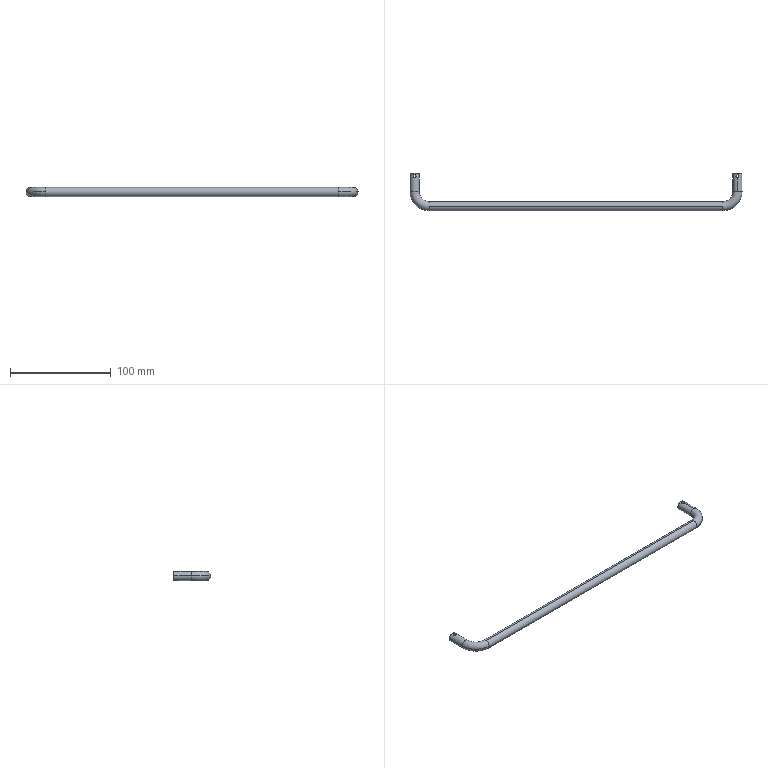Part | SolidWorks | features Chamfer 1, ICE 1, Sweep 1 | 1 solid | 20 faces | box 329 x 37 x 9 mm | volume 23569 mm3 | cylinder 10 | torus 4 | cone 4 | plane 2 | commonest cylinder face diameters 9 x6 3 x4
STEP:
#1=CARTESIAN_POINT('',(-4.5,-18.,0.));
#2=VERTEX_POINT('',#1);
#3=CARTESIAN_POINT('',(4.5,-18.,0.));
#4=VERTEX_POINT('',#3);
#5=CARTESIAN_POINT('',(0.,-18.,0.));
#6=DIRECTION('',(0.,1.,0.));
#7=DIRECTION('',(0.,0.,1.));
#8=AXIS2_PLACEMENT_3D('',#5,#6,#7);
#9=CIRCLE('',#8,4.5);
#10=EDGE_CURVE('',#2,#4,#9,.T.);
#11=ORIENTED_EDGE('',*,*,#10,.F.);
#12=CARTESIAN_POINT('',(14.5,-37.,0.));
#13=VERTEX_POINT('',#12);
#14=CARTESIAN_POINT('',(14.5,-18.,0.));
#15=DIRECTION('',(0.,0.,1.));
#16=DIRECTION('',(1.,0.,0.));
#17=AXIS2_PLACEMENT_3D('',#14,#15,#16);
#18=CIRCLE('',#17,19.);
#19=EDGE_CURVE('',#2,#13,#18,.T.);
#20=ORIENTED_EDGE('',*,*,#19,.T.);
#21=CARTESIAN_POINT('',(14.5,-32.5,4.5));
#22=VERTEX_POINT('',#21);
#23=CARTESIAN_POINT('',(14.5,-32.5,0.));
#24=DIRECTION('',(-1.,0.,0.));
#25=DIRECTION('',(0.,0.,1.));
#26=AXIS2_PLACEMENT_3D('',#23,#24,#25);
#27=CIRCLE('',#26,4.5);
#28=EDGE_CURVE('',#13,#22,#27,.T.);
#29=ORIENTED_EDGE('',*,*,#28,.T.);
#30=CARTESIAN_POINT('',(14.5,-28.,0.));
#31=VERTEX_POINT('',#30);
#32=CARTESIAN_POINT('',(14.5,-32.5,0.));
#33=DIRECTION('',(-1.,0.,0.));
#34=DIRECTION('',(0.,0.,1.));
#35=AXIS2_PLACEMENT_3D('',#32,#33,#34);
#36=CIRCLE('',#35,4.5);
#37=EDGE_CURVE('',#22,#31,#36,.T.);
#38=ORIENTED_EDGE('',*,*,#37,.T.);
#39=CARTESIAN_POINT('',(14.5,-18.,0.));
#40=DIRECTION('',(0.,0.,1.));
#41=DIRECTION('',(1.,0.,0.));
#42=AXIS2_PLACEMENT_3D('',#39,#40,#41);
#43=CIRCLE('',#42,10.);
#44=EDGE_CURVE('',#4,#31,#43,.T.);
#45=ORIENTED_EDGE('',*,*,#44,.F.);
#46=EDGE_LOOP('',(#11,#20,#29,#38,#45));
#47=FACE_OUTER_BOUND('',#46,.T.);
#48=CARTESIAN_POINT('',(14.5,-18.,0.));
#49=DIRECTION('',(0.,0.,1.));
#50=DIRECTION('',(1.,0.,0.));
#51=AXIS2_PLACEMENT_3D('',#48,#49,#50);
#52=TOROIDAL_SURFACE('',#51,14.5,4.5);
#53=ADVANCED_FACE('',(#47),#52,.T.);
#54=CARTESIAN_POINT('',(305.5,-37.,0.));
#55=VERTEX_POINT('',#54);
#56=CARTESIAN_POINT('',(305.5,-32.5,4.5));
#57=VERTEX_POINT('',#56);
#58=CARTESIAN_POINT('',(305.5,-32.5,0.));
#59=DIRECTION('',(-1.,0.,0.));
#60=DIRECTION('',(0.,0.,1.));
#61=AXIS2_PLACEMENT_3D('',#58,#59,#60);
#62=CIRCLE('',#61,4.5);
#63=EDGE_CURVE('',#55,#57,#62,.T.);
#64=ORIENTED_EDGE('',*,*,#63,.F.);
#65=CARTESIAN_POINT('',(324.5,-18.,0.));
#66=VERTEX_POINT('',#65);
#67=CARTESIAN_POINT('',(305.5,-18.,0.));
#68=DIRECTION('',(0.,0.,1.));
#69=DIRECTION('',(1.,0.,0.));
#70=AXIS2_PLACEMENT_3D('',#67,#68,#69);
#71=CIRCLE('',#70,19.);
#72=EDGE_CURVE('',#55,#66,#71,.T.);
#73=ORIENTED_EDGE('',*,*,#72,.T.);
#74=CARTESIAN_POINT('',(320.,-18.,4.5));
#75=VERTEX_POINT('',#74);
#76=CARTESIAN_POINT('',(320.,-18.,0.));
#77=DIRECTION('',(0.,-1.,0.));
#78=DIRECTION('',(0.,0.,1.));
#79=AXIS2_PLACEMENT_3D('',#76,#77,#78);
#80=CIRCLE('',#79,4.5);
#81=EDGE_CURVE('',#66,#75,#80,.T.);
#82=ORIENTED_EDGE('',*,*,#81,.T.);
#83=CARTESIAN_POINT('',(315.5,-18.,0.));
#84=VERTEX_POINT('',#83);
#85=CARTESIAN_POINT('',(320.,-18.,0.));
#86=DIRECTION('',(0.,-1.,0.));
#87=DIRECTION('',(0.,0.,1.));
#88=AXIS2_PLACEMENT_3D('',#85,#86,#87);
#89=CIRCLE('',#88,4.5);
#90=EDGE_CURVE('',#75,#84,#89,.T.);
#91=ORIENTED_EDGE('',*,*,#90,.T.);
#92=CARTESIAN_POINT('',(305.5,-28.,0.));
#93=VERTEX_POINT('',#92);
#94=CARTESIAN_POINT('',(305.5,-18.,0.));
#95=DIRECTION('',(0.,0.,1.));
#96=DIRECTION('',(1.,0.,0.));
#97=AXIS2_PLACEMENT_3D('',#94,#95,#96);
#98=CIRCLE('',#97,10.);
#99=EDGE_CURVE('',#93,#84,#98,.T.);
#100=ORIENTED_EDGE('',*,*,#99,.F.);
#101=CARTESIAN_POINT('',(305.5,-32.5,0.));
#102=DIRECTION('',(-1.,0.,0.));
#103=DIRECTION('',(0.,0.,1.));
#104=AXIS2_PLACEMENT_3D('',#101,#102,#103);
#105=CIRCLE('',#104,4.5);
#106=EDGE_CURVE('',#57,#93,#105,.T.);
#107=ORIENTED_EDGE('',*,*,#106,.F.);
#108=EDGE_LOOP('',(#64,#73,#82,#91,#100,#107));
#109=FACE_OUTER_BOUND('',#108,.T.);
#110=CARTESIAN_POINT('',(305.5,-18.,0.));
#111=DIRECTION('',(0.,0.,1.));
#112=DIRECTION('',(1.,0.,0.));
#113=AXIS2_PLACEMENT_3D('',#110,#111,#112);
#114=TOROIDAL_SURFACE('',#113,14.5,4.5);
#115=ADVANCED_FACE('',(#109),#114,.T.);
#116=CARTESIAN_POINT('',(-4.,0.,0.));
#117=VERTEX_POINT('',#116);
#118=CARTESIAN_POINT('',(4.,0.,0.));
#119=VERTEX_POINT('',#118);
#120=CARTESIAN_POINT('',(0.,0.,0.));
#121=DIRECTION('',(0.,1.,0.));
#122=DIRECTION('',(0.,0.,1.));
#123=AXIS2_PLACEMENT_3D('',#120,#121,#122);
#124=CIRCLE('',#123,4.);
#125=EDGE_CURVE('',#117,#119,#124,.T.);
#126=ORIENTED_EDGE('',*,*,#125,.F.);
#127=CARTESIAN_POINT('',(-4.5,-0.5,0.));
#128=VERTEX_POINT('',#127);
#129=CARTESIAN_POINT('',(-4.,0.,0.));
#130=DIRECTION('',(-0.7071,-0.7071,0.));
#131=VECTOR('',#130,1000.);
#132=LINE('',#129,#131);
#133=EDGE_CURVE('',#117,#128,#132,.T.);
#134=ORIENTED_EDGE('',*,*,#133,.T.);
#135=CARTESIAN_POINT('',(4.5,-0.5,0.));
#136=VERTEX_POINT('',#135);
#137=CARTESIAN_POINT('',(0.,-0.5,0.));
#138=DIRECTION('',(0.,-1.,0.));
#139=DIRECTION('',(-1.,0.,0.));
#140=AXIS2_PLACEMENT_3D('',#137,#138,#139);
#141=CIRCLE('',#140,4.5);
#142=EDGE_CURVE('',#136,#128,#141,.T.);
#143=ORIENTED_EDGE('',*,*,#142,.F.);
#144=CARTESIAN_POINT('',(4.,0.,0.));
#145=DIRECTION('',(0.7071,-0.7071,0.));
#146=VECTOR('',#145,1000.);
#147=LINE('',#144,#146);
#148=EDGE_CURVE('',#119,#136,#147,.T.);
#149=ORIENTED_EDGE('',*,*,#148,.F.);
#150=EDGE_LOOP('',(#126,#134,#143,#149));
#151=FACE_OUTER_BOUND('',#150,.T.);
#152=CARTESIAN_POINT('',(0.,0.,0.));
#153=DIRECTION('',(0.,-1.,0.));
#154=DIRECTION('',(1.,0.,0.));
#155=AXIS2_PLACEMENT_3D('',#152,#153,#154);
#156=CONICAL_SURFACE('',#155,4.,0.7854);
#157=ADVANCED_FACE('',(#151),#156,.T.);
#158=CARTESIAN_POINT('',(320.,0.,4.));
#159=VERTEX_POINT('',#158);
#160=CARTESIAN_POINT('',(320.,0.,-4.));
#161=VERTEX_POINT('',#160);
#162=CARTESIAN_POINT('',(320.,0.,0.));
#163=DIRECTION('',(0.,1.,0.));
#164=DIRECTION('',(1.,0.,0.));
#165=AXIS2_PLACEMENT_3D('',#162,#163,#164);
#166=CIRCLE('',#165,4.);
#167=EDGE_CURVE('',#159,#161,#166,.T.);
#168=ORIENTED_EDGE('',*,*,#167,.F.);
#169=CARTESIAN_POINT('',(320.,-0.5,4.5));
#170=VERTEX_POINT('',#169);
#171=CARTESIAN_POINT('',(320.,-0.5,4.5));
#172=DIRECTION('',(0.,-0.7071,0.7071));
#173=VECTOR('',#172,1000.);
#174=LINE('',#171,#173);
#175=EDGE_CURVE('',#159,#170,#174,.T.);
#176=ORIENTED_EDGE('',*,*,#175,.T.);
#177=CARTESIAN_POINT('',(320.,-0.5,-4.5));
#178=VERTEX_POINT('',#177);
#179=CARTESIAN_POINT('',(320.,-0.5,0.));
#180=DIRECTION('',(0.,-1.,0.));
#181=DIRECTION('',(0.,0.,-1.));
#182=AXIS2_PLACEMENT_3D('',#179,#180,#181);
#183=CIRCLE('',#182,4.5);
#184=EDGE_CURVE('',#178,#170,#183,.T.);
#185=ORIENTED_EDGE('',*,*,#184,.F.);
#186=CARTESIAN_POINT('',(320.,-0.5,-4.5));
#187=DIRECTION('',(0.,-0.7071,-0.7071));
#188=VECTOR('',#187,1000.);
#189=LINE('',#186,#188);
#190=EDGE_CURVE('',#161,#178,#189,.T.);
#191=ORIENTED_EDGE('',*,*,#190,.F.);
#192=EDGE_LOOP('',(#168,#176,#185,#191));
#193=FACE_OUTER_BOUND('',#192,.T.);
#194=CARTESIAN_POINT('',(320.,-0.5,0.));
#195=DIRECTION('',(0.,-1.,0.));
#196=DIRECTION('',(0.,0.,-1.));
#197=AXIS2_PLACEMENT_3D('',#194,#195,#196);
#198=CONICAL_SURFACE('',#197,4.5,0.7854);
#199=ADVANCED_FACE('',(#193),#198,.T.);
#200=CARTESIAN_POINT('',(1.5,-3.,4.243));
#201=VERTEX_POINT('',#200);
#202=CARTESIAN_POINT('',(-1.5,-3.,4.243));
#203=VERTEX_POINT('',#202);
#204=CARTESIAN_POINT('',(1.5,-3.,4.243));
#205=CARTESIAN_POINT('',(1.5,-3.197,4.243));
#206=CARTESIAN_POINT('',(1.46,-3.395,4.257));
#207=CARTESIAN_POINT('',(1.347,-3.667,4.294));
#208=CARTESIAN_POINT('',(1.3,-3.754,4.308));
#209=CARTESIAN_POINT('',(1.192,-3.916,4.34));
#210=CARTESIAN_POINT('',(1.13,-3.991,4.356));
#211=CARTESIAN_POINT('',(0.9222,-4.199,4.407));
#212=CARTESIAN_POINT('',(0.7586,-4.309,4.439));
#213=CARTESIAN_POINT('',(0.485,-4.423,4.475));
#214=CARTESIAN_POINT('',(0.3913,-4.451,4.484));
#215=CARTESIAN_POINT('',(0.1987,-4.49,4.497));
#216=CARTESIAN_POINT('',(0.09861,-4.5,4.5));
#217=CARTESIAN_POINT('',(-0.09905,-4.5,4.5));
#218=CARTESIAN_POINT('',(-0.1969,-4.49,4.497));
#219=CARTESIAN_POINT('',(-0.3908,-4.452,4.484));
#220=CARTESIAN_POINT('',(-0.4863,-4.422,4.475));
#221=CARTESIAN_POINT('',(-0.7573,-4.31,4.44));
#222=CARTESIAN_POINT('',(-0.9233,-4.198,4.407));
#223=CARTESIAN_POINT('',(-1.13,-3.992,4.357));
#224=CARTESIAN_POINT('',(-1.192,-3.915,4.34));
#225=CARTESIAN_POINT('',(-1.301,-3.753,4.308));
#226=CARTESIAN_POINT('',(-1.347,-3.667,4.294));
#227=CARTESIAN_POINT('',(-1.422,-3.486,4.269));
#228=CARTESIAN_POINT('',(-1.452,-3.391,4.259));
#229=CARTESIAN_POINT('',(-1.49,-3.198,4.246));
#230=CARTESIAN_POINT('',(-1.5,-3.1,4.243));
#231=CARTESIAN_POINT('',(-1.5,-3.,4.243));
#232=B_SPLINE_CURVE_WITH_KNOTS('',3,(#204,#205,#206,#207,#208,#209,#210,#211,#212,#213,#214,#215,#216,#217,#218,#219,#220,#221,#222,#223,#224,#225,#226,#227,#228,#229,#230,#231),.UNSPECIFIED.,.F.,.F.,(4,2,2,2,2,2,2,2,2,2,2,2,2,4),(0.004724,0.005314,0.005609,0.005904,0.006495,0.00679,0.007085,0.00738,0.007675,0.008265,0.008561,0.008856,0.009151,0.009446),.UNSPECIFIED.);
#233=EDGE_CURVE('',#201,#203,#232,.T.);
#234=ORIENTED_EDGE('',*,*,#233,.F.);
#235=CARTESIAN_POINT('',(1.5,-3.,-4.243));
#236=VERTEX_POINT('',#235);
#237=CARTESIAN_POINT('',(1.5,-3.,10.));
#238=DIRECTION('',(0.,0.,-1.));
#239=VECTOR('',#238,1000.);
#240=LINE('',#237,#239);
#241=EDGE_CURVE('',#201,#236,#240,.T.);
#242=ORIENTED_EDGE('',*,*,#241,.T.);
#243=CARTESIAN_POINT('',(-1.5,-3.,-4.243));
#244=VERTEX_POINT('',#243);
#245=CARTESIAN_POINT('',(-1.5,-3.,-4.243));
#246=CARTESIAN_POINT('',(-1.5,-3.1,-4.243));
#247=CARTESIAN_POINT('',(-1.49,-3.198,-4.246));
#248=CARTESIAN_POINT('',(-1.452,-3.391,-4.26));
#249=CARTESIAN_POINT('',(-1.422,-3.486,-4.269));
#250=CARTESIAN_POINT('',(-1.309,-3.758,-4.306));
#251=CARTESIAN_POINT('',(-1.198,-3.924,-4.34));
#252=CARTESIAN_POINT('',(-0.9231,-4.198,-4.407));
#253=CARTESIAN_POINT('',(-0.757,-4.31,-4.44));
#254=CARTESIAN_POINT('',(-0.3964,-4.46,-4.486));
#255=CARTESIAN_POINT('',(-0.198,-4.5,-4.5));
#256=CARTESIAN_POINT('',(0.09798,-4.5,-4.5));
#257=CARTESIAN_POINT('',(0.1982,-4.49,-4.497));
#258=CARTESIAN_POINT('',(0.3912,-4.451,-4.484));
#259=CARTESIAN_POINT('',(0.4851,-4.423,-4.475));
#260=CARTESIAN_POINT('',(0.759,-4.309,-4.439));
#261=CARTESIAN_POINT('',(0.9234,-4.198,-4.407));
#262=CARTESIAN_POINT('',(1.13,-3.991,-4.356));
#263=CARTESIAN_POINT('',(1.192,-3.916,-4.34));
#264=CARTESIAN_POINT('',(1.3,-3.754,-4.308));
#265=CARTESIAN_POINT('',(1.348,-3.666,-4.294));
#266=CARTESIAN_POINT('',(1.46,-3.395,-4.257));
#267=CARTESIAN_POINT('',(1.5,-3.197,-4.243));
#268=CARTESIAN_POINT('',(1.5,-3.,-4.243));
#269=B_SPLINE_CURVE_WITH_KNOTS('',3,(#245,#246,#247,#248,#249,#250,#251,#252,#253,#254,#255,#256,#257,#258,#259,#260,#261,#262,#263,#264,#265,#266,#267,#268),.UNSPECIFIED.,.F.,.F.,(4,2,2,2,2,2,2,2,2,2,2,4),(0.,0.0002952,0.0005905,0.001181,0.001771,0.002362,0.002657,0.002952,0.003543,0.003838,0.004133,0.004724),.UNSPECIFIED.);
#270=EDGE_CURVE('',#244,#236,#269,.T.);
#271=ORIENTED_EDGE('',*,*,#270,.F.);
#272=CARTESIAN_POINT('',(-1.5,-3.,10.));
#273=DIRECTION('',(0.,0.,-1.));
#274=VECTOR('',#273,1000.);
#275=LINE('',#272,#274);
#276=EDGE_CURVE('',#203,#244,#275,.T.);
#277=ORIENTED_EDGE('',*,*,#276,.F.);
#278=EDGE_LOOP('',(#234,#242,#271,#277));
#279=FACE_OUTER_BOUND('',#278,.T.);
#280=CARTESIAN_POINT('',(0.,-3.,10.));
#281=DIRECTION('',(0.,0.,-1.));
#282=DIRECTION('',(-1.,0.,0.));
#283=AXIS2_PLACEMENT_3D('',#280,#281,#282);
#284=CYLINDRICAL_SURFACE('',#283,1.5);
#285=ADVANCED_FACE('',(#279),#284,.F.);
#286=CARTESIAN_POINT('',(320.,-4.5,4.5));
#287=VERTEX_POINT('',#286);
#288=CARTESIAN_POINT('',(321.5,-3.,4.243));
#289=VERTEX_POINT('',#288);
#290=CARTESIAN_POINT('',(320.,-4.5,4.5));
#291=CARTESIAN_POINT('',(320.1,-4.5,4.5));
#292=CARTESIAN_POINT('',(320.198,-4.49,4.497));
#293=CARTESIAN_POINT('',(320.391,-4.452,4.484));
#294=CARTESIAN_POINT('',(320.486,-4.422,4.475));
#295=CARTESIAN_POINT('',(320.759,-4.309,4.439));
#296=CARTESIAN_POINT('',(320.924,-4.197,4.406));
#297=CARTESIAN_POINT('',(321.199,-3.922,4.34));
#298=CARTESIAN_POINT('',(321.31,-3.756,4.306));
#299=CARTESIAN_POINT('',(321.46,-3.396,4.257));
#300=CARTESIAN_POINT('',(321.5,-3.197,4.243));
#301=CARTESIAN_POINT('',(321.5,-3.,4.243));
#302=B_SPLINE_CURVE_WITH_KNOTS('',3,(#290,#291,#292,#293,#294,#295,#296,#297,#298,#299,#300,#301),.UNSPECIFIED.,.F.,.F.,(4,2,2,2,2,4),(0.,0.0002953,0.0005907,0.001181,0.001772,0.002363),.UNSPECIFIED.);
#303=EDGE_CURVE('',#287,#289,#302,.T.);
#304=ORIENTED_EDGE('',*,*,#303,.T.);
#305=CARTESIAN_POINT('',(321.5,-3.,-4.243));
#306=VERTEX_POINT('',#305);
#307=CARTESIAN_POINT('',(321.5,-3.,10.));
#308=DIRECTION('',(0.,0.,-1.));
#309=VECTOR('',#308,1000.);
#310=LINE('',#307,#309);
#311=EDGE_CURVE('',#289,#306,#310,.T.);
#312=ORIENTED_EDGE('',*,*,#311,.T.);
#313=CARTESIAN_POINT('',(320.,-4.5,-4.5));
#314=VERTEX_POINT('',#313);
#315=CARTESIAN_POINT('',(321.5,-3.,-4.243));
#316=CARTESIAN_POINT('',(321.5,-3.197,-4.243));
#317=CARTESIAN_POINT('',(321.46,-3.395,-4.257));
#318=CARTESIAN_POINT('',(321.347,-3.667,-4.294));
#319=CARTESIAN_POINT('',(321.3,-3.754,-4.308));
#320=CARTESIAN_POINT('',(321.192,-3.916,-4.34));
#321=CARTESIAN_POINT('',(321.13,-3.991,-4.356));
#322=CARTESIAN_POINT('',(320.922,-4.199,-4.407));
#323=CARTESIAN_POINT('',(320.759,-4.309,-4.439));
#324=CARTESIAN_POINT('',(320.485,-4.423,-4.475));
#325=CARTESIAN_POINT('',(320.391,-4.451,-4.484));
#326=CARTESIAN_POINT('',(320.199,-4.49,-4.497));
#327=CARTESIAN_POINT('',(320.099,-4.5,-4.5));
#328=CARTESIAN_POINT('',(320.,-4.5,-4.5));
#329=B_SPLINE_CURVE_WITH_KNOTS('',3,(#315,#316,#317,#318,#319,#320,#321,#322,#323,#324,#325,#326,#327,#328),.UNSPECIFIED.,.F.,.F.,(4,2,2,2,2,2,4),(0.004724,0.005314,0.005609,0.005904,0.006494,0.006789,0.007085),.UNSPECIFIED.);
#330=EDGE_CURVE('',#306,#314,#329,.T.);
#331=ORIENTED_EDGE('',*,*,#330,.T.);
#332=CARTESIAN_POINT('',(318.5,-3.,-4.243));
#333=VERTEX_POINT('',#332);
#334=CARTESIAN_POINT('',(320.,-4.5,-4.5));
#335=CARTESIAN_POINT('',(319.901,-4.5,-4.5));
#336=CARTESIAN_POINT('',(319.803,-4.49,-4.497));
#337=CARTESIAN_POINT('',(319.609,-4.452,-4.484));
#338=CARTESIAN_POINT('',(319.514,-4.422,-4.475));
#339=CARTESIAN_POINT('',(319.243,-4.31,-4.44));
#340=CARTESIAN_POINT('',(319.077,-4.198,-4.407));
#341=CARTESIAN_POINT('',(318.871,-3.992,-4.357));
#342=CARTESIAN_POINT('',(318.808,-3.915,-4.34));
#343=CARTESIAN_POINT('',(318.699,-3.753,-4.308));
#344=CARTESIAN_POINT('',(318.653,-3.667,-4.294));
#345=CARTESIAN_POINT('',(318.578,-3.486,-4.269));
#346=CARTESIAN_POINT('',(318.548,-3.391,-4.259));
#347=CARTESIAN_POINT('',(318.51,-3.198,-4.246));
#348=CARTESIAN_POINT('',(318.5,-3.1,-4.243));
#349=CARTESIAN_POINT('',(318.5,-3.,-4.243));
#350=B_SPLINE_CURVE_WITH_KNOTS('',3,(#334,#335,#336,#337,#338,#339,#340,#341,#342,#343,#344,#345,#346,#347,#348,#349),.UNSPECIFIED.,.F.,.F.,(4,2,2,2,2,2,2,4),(0.007085,0.00738,0.007675,0.008265,0.00856,0.008856,0.009151,0.009446),.UNSPECIFIED.);
#351=EDGE_CURVE('',#314,#333,#350,.T.);
#352=ORIENTED_EDGE('',*,*,#351,.T.);
#353=CARTESIAN_POINT('',(318.5,-3.,4.243));
#354=VERTEX_POINT('',#353);
#355=CARTESIAN_POINT('',(318.5,-3.,10.));
#356=DIRECTION('',(0.,0.,-1.));
#357=VECTOR('',#356,1000.);
#358=LINE('',#355,#357);
#359=EDGE_CURVE('',#354,#333,#358,.T.);
#360=ORIENTED_EDGE('',*,*,#359,.F.);
#361=CARTESIAN_POINT('',(318.5,-3.,4.243));
#362=CARTESIAN_POINT('',(318.5,-3.099,4.243));
#363=CARTESIAN_POINT('',(318.51,-3.197,4.246));
#364=CARTESIAN_POINT('',(318.548,-3.391,4.259));
#365=CARTESIAN_POINT('',(318.578,-3.486,4.269));
#366=CARTESIAN_POINT('',(318.69,-3.757,4.306));
#367=CARTESIAN_POINT('',(318.802,-3.923,4.34));
#368=CARTESIAN_POINT('',(319.008,-4.129,4.39));
#369=CARTESIAN_POINT('',(319.084,-4.192,4.407));
#370=CARTESIAN_POINT('',(319.247,-4.301,4.437));
#371=CARTESIAN_POINT('',(319.332,-4.347,4.451));
#372=CARTESIAN_POINT('',(319.514,-4.422,4.475));
#373=CARTESIAN_POINT('',(319.609,-4.452,4.484));
#374=CARTESIAN_POINT('',(319.802,-4.49,4.497));
#375=CARTESIAN_POINT('',(319.9,-4.5,4.5));
#376=CARTESIAN_POINT('',(320.,-4.5,4.5));
#377=B_SPLINE_CURVE_WITH_KNOTS('',3,(#361,#362,#363,#364,#365,#366,#367,#368,#369,#370,#371,#372,#373,#374,#375,#376),.UNSPECIFIED.,.F.,.F.,(4,2,2,2,2,2,2,4),(0.007085,0.00738,0.007675,0.008266,0.008561,0.008856,0.009151,0.009446),.UNSPECIFIED.);
#378=EDGE_CURVE('',#354,#287,#377,.T.);
#379=ORIENTED_EDGE('',*,*,#378,.T.);
#380=EDGE_LOOP('',(#304,#312,#331,#352,#360,#379));
#381=FACE_OUTER_BOUND('',#380,.T.);
#382=CARTESIAN_POINT('',(320.,-3.,10.));
#383=DIRECTION('',(0.,0.,-1.));
#384=DIRECTION('',(-1.,0.,0.));
#385=AXIS2_PLACEMENT_3D('',#382,#383,#384);
#386=CYLINDRICAL_SURFACE('',#385,1.5);
#387=ADVANCED_FACE('',(#381),#386,.F.);
#388=ORIENTED_EDGE('',*,*,#37,.F.);
#389=CARTESIAN_POINT('',(14.5,-32.5,4.5));
#390=DIRECTION('',(1.,0.,0.));
#391=VECTOR('',#390,1000.);
#392=LINE('',#389,#391);
#393=EDGE_CURVE('',#22,#57,#392,.T.);
#394=ORIENTED_EDGE('',*,*,#393,.T.);
#395=ORIENTED_EDGE('',*,*,#106,.T.);
#396=CARTESIAN_POINT('',(305.5,-32.5,-4.5));
#397=VERTEX_POINT('',#396);
#398=CARTESIAN_POINT('',(305.5,-32.5,0.));
#399=DIRECTION('',(-1.,0.,0.));
#400=DIRECTION('',(0.,0.,1.));
#401=AXIS2_PLACEMENT_3D('',#398,#399,#400);
#402=CIRCLE('',#401,4.5);
#403=EDGE_CURVE('',#93,#397,#402,.T.);
#404=ORIENTED_EDGE('',*,*,#403,.T.);
#405=CARTESIAN_POINT('',(14.5,-32.5,-4.5));
#406=VERTEX_POINT('',#405);
#407=CARTESIAN_POINT('',(14.5,-32.5,-4.5));
#408=DIRECTION('',(1.,0.,0.));
#409=VECTOR('',#408,1000.);
#410=LINE('',#407,#409);
#411=EDGE_CURVE('',#406,#397,#410,.T.);
#412=ORIENTED_EDGE('',*,*,#411,.F.);
#413=CARTESIAN_POINT('',(14.5,-32.5,0.));
#414=DIRECTION('',(-1.,0.,0.));
#415=DIRECTION('',(0.,0.,1.));
#416=AXIS2_PLACEMENT_3D('',#413,#414,#415);
#417=CIRCLE('',#416,4.5);
#418=EDGE_CURVE('',#31,#406,#417,.T.);
#419=ORIENTED_EDGE('',*,*,#418,.F.);
#420=EDGE_LOOP('',(#388,#394,#395,#404,#412,#419));
#421=FACE_OUTER_BOUND('',#420,.T.);
#422=CARTESIAN_POINT('',(14.5,-32.5,0.));
#423=DIRECTION('',(1.,0.,0.));
#424=DIRECTION('',(0.,0.,-1.));
#425=AXIS2_PLACEMENT_3D('',#422,#423,#424);
#426=CYLINDRICAL_SURFACE('',#425,4.5);
#427=ADVANCED_FACE('',(#421),#426,.T.);
#428=CARTESIAN_POINT('',(320.,-18.,-4.5));
#429=VERTEX_POINT('',#428);
#430=CARTESIAN_POINT('',(320.,-18.,0.));
#431=DIRECTION('',(0.,-1.,0.));
#432=DIRECTION('',(0.,0.,1.));
#433=AXIS2_PLACEMENT_3D('',#430,#431,#432);
#434=CIRCLE('',#433,4.5);
#435=EDGE_CURVE('',#429,#66,#434,.T.);
#436=ORIENTED_EDGE('',*,*,#435,.F.);
#437=CARTESIAN_POINT('',(320.,-18.,-4.5));
#438=DIRECTION('',(0.,1.,0.));
#439=VECTOR('',#438,1000.);
#440=LINE('',#437,#439);
#441=EDGE_CURVE('',#429,#314,#440,.T.);
#442=ORIENTED_EDGE('',*,*,#441,.T.);
#443=ORIENTED_EDGE('',*,*,#330,.F.);
#444=CARTESIAN_POINT('',(320.,-1.5,-4.5));
#445=VERTEX_POINT('',#444);
#446=CARTESIAN_POINT('',(320.,-1.5,-4.5));
#447=CARTESIAN_POINT('',(320.099,-1.5,-4.5));
#448=CARTESIAN_POINT('',(320.199,-1.51,-4.497));
#449=CARTESIAN_POINT('',(320.392,-1.549,-4.484));
#450=CARTESIAN_POINT('',(320.486,-1.577,-4.475));
#451=CARTESIAN_POINT('',(320.759,-1.691,-4.439));
#452=CARTESIAN_POINT('',(320.924,-1.802,-4.406));
#453=CARTESIAN_POINT('',(321.131,-2.009,-4.356));
#454=CARTESIAN_POINT('',(321.192,-2.084,-4.34));
#455=CARTESIAN_POINT('',(321.301,-2.246,-4.308));
#456=CARTESIAN_POINT('',(321.348,-2.334,-4.294));
#457=CARTESIAN_POINT('',(321.46,-2.605,-4.257));
#458=CARTESIAN_POINT('',(321.5,-2.803,-4.243));
#459=CARTESIAN_POINT('',(321.5,-3.,-4.243));
#460=B_SPLINE_CURVE_WITH_KNOTS('',3,(#446,#447,#448,#449,#450,#451,#452,#453,#454,#455,#456,#457,#458,#459),.UNSPECIFIED.,.F.,.F.,(4,2,2,2,2,2,4),(0.002362,0.002658,0.002953,0.003543,0.003838,0.004133,0.004724),.UNSPECIFIED.);
#461=EDGE_CURVE('',#445,#306,#460,.T.);
#462=ORIENTED_EDGE('',*,*,#461,.F.);
#463=CARTESIAN_POINT('',(320.,-18.,-4.5));
#464=DIRECTION('',(0.,1.,0.));
#465=VECTOR('',#464,1000.);
#466=LINE('',#463,#465);
#467=EDGE_CURVE('',#445,#178,#466,.T.);
#468=ORIENTED_EDGE('',*,*,#467,.T.);
#469=ORIENTED_EDGE('',*,*,#184,.T.);
#470=CARTESIAN_POINT('',(320.,-1.5,4.5));
#471=VERTEX_POINT('',#470);
#472=CARTESIAN_POINT('',(320.,-18.,4.5));
#473=DIRECTION('',(0.,1.,0.));
#474=VECTOR('',#473,1000.);
#475=LINE('',#472,#474);
#476=EDGE_CURVE('',#471,#170,#475,.T.);
#477=ORIENTED_EDGE('',*,*,#476,.F.);
#478=CARTESIAN_POINT('',(321.5,-3.,4.243));
#479=CARTESIAN_POINT('',(321.5,-2.901,4.243));
#480=CARTESIAN_POINT('',(321.49,-2.801,4.246));
#481=CARTESIAN_POINT('',(321.451,-2.608,4.26));
#482=CARTESIAN_POINT('',(321.423,-2.514,4.269));
#483=CARTESIAN_POINT('',(321.309,-2.241,4.306));
#484=CARTESIAN_POINT('',(321.198,-2.077,4.34));
#485=CARTESIAN_POINT('',(320.991,-1.87,4.39));
#486=CARTESIAN_POINT('',(320.916,-1.808,4.407));
#487=CARTESIAN_POINT('',(320.754,-1.7,4.437));
#488=CARTESIAN_POINT('',(320.666,-1.652,4.451));
#489=CARTESIAN_POINT('',(320.395,-1.54,4.486));
#490=CARTESIAN_POINT('',(320.197,-1.5,4.5));
#491=CARTESIAN_POINT('',(320.,-1.5,4.5));
#492=B_SPLINE_CURVE_WITH_KNOTS('',3,(#478,#479,#480,#481,#482,#483,#484,#485,#486,#487,#488,#489,#490,#491),.UNSPECIFIED.,.F.,.F.,(4,2,2,2,2,2,4),(0.002363,0.002658,0.002953,0.003543,0.003838,0.004133,0.004724),.UNSPECIFIED.);
#493=EDGE_CURVE('',#289,#471,#492,.T.);
#494=ORIENTED_EDGE('',*,*,#493,.F.);
#495=ORIENTED_EDGE('',*,*,#303,.F.);
#496=CARTESIAN_POINT('',(320.,-18.,4.5));
#497=DIRECTION('',(0.,1.,0.));
#498=VECTOR('',#497,1000.);
#499=LINE('',#496,#498);
#500=EDGE_CURVE('',#75,#287,#499,.T.);
#501=ORIENTED_EDGE('',*,*,#500,.F.);
#502=ORIENTED_EDGE('',*,*,#81,.F.);
#503=EDGE_LOOP('',(#436,#442,#443,#462,#468,#469,#477,#494,#495,#501,#502));
#504=FACE_OUTER_BOUND('',#503,.T.);
#505=CARTESIAN_POINT('',(320.,-18.,0.));
#506=DIRECTION('',(0.,1.,0.));
#507=DIRECTION('',(0.,0.,1.));
#508=AXIS2_PLACEMENT_3D('',#505,#506,#507);
#509=CYLINDRICAL_SURFACE('',#508,4.5);
#510=ADVANCED_FACE('',(#504),#509,.T.);
#511=CARTESIAN_POINT('',(-1.5,-3.,4.243));
#512=CARTESIAN_POINT('',(-1.5,-2.9,4.243));
#513=CARTESIAN_POINT('',(-1.49,-2.802,4.246));
#514=CARTESIAN_POINT('',(-1.452,-2.609,4.26));
#515=CARTESIAN_POINT('',(-1.422,-2.514,4.269));
#516=CARTESIAN_POINT('',(-1.309,-2.242,4.306));
#517=CARTESIAN_POINT('',(-1.198,-2.076,4.34));
#518=CARTESIAN_POINT('',(-0.9231,-1.802,4.407));
#519=CARTESIAN_POINT('',(-0.757,-1.69,4.44));
#520=CARTESIAN_POINT('',(-0.3964,-1.54,4.486));
#521=CARTESIAN_POINT('',(-0.198,-1.5,4.5));
#522=CARTESIAN_POINT('',(0.09798,-1.5,4.5));
#523=CARTESIAN_POINT('',(0.1982,-1.51,4.497));
#524=CARTESIAN_POINT('',(0.3912,-1.549,4.484));
#525=CARTESIAN_POINT('',(0.4851,-1.577,4.475));
#526=CARTESIAN_POINT('',(0.759,-1.691,4.439));
#527=CARTESIAN_POINT('',(0.9234,-1.802,4.407));
#528=CARTESIAN_POINT('',(1.13,-2.009,4.356));
#529=CARTESIAN_POINT('',(1.192,-2.084,4.34));
#530=CARTESIAN_POINT('',(1.3,-2.246,4.308));
#531=CARTESIAN_POINT('',(1.348,-2.334,4.294));
#532=CARTESIAN_POINT('',(1.46,-2.605,4.257));
#533=CARTESIAN_POINT('',(1.5,-2.803,4.243));
#534=CARTESIAN_POINT('',(1.5,-3.,4.243));
#535=B_SPLINE_CURVE_WITH_KNOTS('',3,(#511,#512,#513,#514,#515,#516,#517,#518,#519,#520,#521,#522,#523,#524,#525,#526,#527,#528,#529,#530,#531,#532,#533,#534),.UNSPECIFIED.,.F.,.F.,(4,2,2,2,2,2,2,2,2,2,2,4),(0.,0.0002952,0.0005905,0.001181,0.001771,0.002362,0.002657,0.002952,0.003543,0.003838,0.004133,0.004724),.UNSPECIFIED.);
#536=EDGE_CURVE('',#203,#201,#535,.T.);
#537=ORIENTED_EDGE('',*,*,#536,.T.);
#538=ORIENTED_EDGE('',*,*,#233,.T.);
#539=EDGE_LOOP('',(#537,#538));
#540=FACE_BOUND('',#539,.T.);
#541=ORIENTED_EDGE('',*,*,#10,.T.);
#542=CARTESIAN_POINT('',(4.5,-18.,0.));
#543=DIRECTION('',(0.,1.,0.));
#544=VECTOR('',#543,1000.);
#545=LINE('',#542,#544);
#546=EDGE_CURVE('',#4,#136,#545,.T.);
#547=ORIENTED_EDGE('',*,*,#546,.T.);
#548=ORIENTED_EDGE('',*,*,#142,.T.);
#549=CARTESIAN_POINT('',(-4.5,-18.,0.));
#550=DIRECTION('',(0.,1.,0.));
#551=VECTOR('',#550,1000.);
#552=LINE('',#549,#551);
#553=EDGE_CURVE('',#2,#128,#552,.T.);
#554=ORIENTED_EDGE('',*,*,#553,.F.);
#555=EDGE_LOOP('',(#541,#547,#548,#554));
#556=FACE_OUTER_BOUND('',#555,.T.);
#557=CARTESIAN_POINT('',(0.,-18.,0.));
#558=DIRECTION('',(0.,1.,0.));
#559=DIRECTION('',(-1.,0.,0.));
#560=AXIS2_PLACEMENT_3D('',#557,#558,#559);
#561=CYLINDRICAL_SURFACE('',#560,4.5);
#562=ADVANCED_FACE('',(#540,#556),#561,.T.);
#563=ORIENTED_EDGE('',*,*,#546,.F.);
#564=CARTESIAN_POINT('',(0.,-18.,0.));
#565=DIRECTION('',(0.,1.,0.));
#566=DIRECTION('',(0.,0.,1.));
#567=AXIS2_PLACEMENT_3D('',#564,#565,#566);
#568=CIRCLE('',#567,4.5);
#569=EDGE_CURVE('',#4,#2,#568,.T.);
#570=ORIENTED_EDGE('',*,*,#569,.T.);
#571=ORIENTED_EDGE('',*,*,#553,.T.);
#572=CARTESIAN_POINT('',(0.,-0.5,0.));
#573=DIRECTION('',(0.,-1.,0.));
#574=DIRECTION('',(-1.,0.,0.));
#575=AXIS2_PLACEMENT_3D('',#572,#573,#574);
#576=CIRCLE('',#575,4.5);
#577=EDGE_CURVE('',#128,#136,#576,.T.);
#578=ORIENTED_EDGE('',*,*,#577,.T.);
#579=EDGE_LOOP('',(#563,#570,#571,#578));
#580=FACE_OUTER_BOUND('',#579,.T.);
#581=ORIENTED_EDGE('',*,*,#270,.T.);
#582=CARTESIAN_POINT('',(1.5,-3.,-4.243));
#583=CARTESIAN_POINT('',(1.5,-2.803,-4.243));
#584=CARTESIAN_POINT('',(1.46,-2.605,-4.257));
#585=CARTESIAN_POINT('',(1.347,-2.333,-4.294));
#586=CARTESIAN_POINT('',(1.3,-2.246,-4.308));
#587=CARTESIAN_POINT('',(1.192,-2.084,-4.34));
#588=CARTESIAN_POINT('',(1.13,-2.009,-4.356));
#589=CARTESIAN_POINT('',(0.9222,-1.801,-4.407));
#590=CARTESIAN_POINT('',(0.7586,-1.691,-4.439));
#591=CARTESIAN_POINT('',(0.485,-1.577,-4.475));
#592=CARTESIAN_POINT('',(0.3913,-1.549,-4.484));
#593=CARTESIAN_POINT('',(0.1987,-1.51,-4.497));
#594=CARTESIAN_POINT('',(0.09861,-1.5,-4.5));
#595=CARTESIAN_POINT('',(-0.09905,-1.5,-4.5));
#596=CARTESIAN_POINT('',(-0.1969,-1.51,-4.497));
#597=CARTESIAN_POINT('',(-0.3908,-1.548,-4.484));
#598=CARTESIAN_POINT('',(-0.4863,-1.578,-4.475));
#599=CARTESIAN_POINT('',(-0.7573,-1.69,-4.44));
#600=CARTESIAN_POINT('',(-0.9233,-1.802,-4.407));
#601=CARTESIAN_POINT('',(-1.13,-2.008,-4.357));
#602=CARTESIAN_POINT('',(-1.192,-2.085,-4.34));
#603=CARTESIAN_POINT('',(-1.301,-2.247,-4.308));
#604=CARTESIAN_POINT('',(-1.347,-2.333,-4.294));
#605=CARTESIAN_POINT('',(-1.422,-2.514,-4.269));
#606=CARTESIAN_POINT('',(-1.452,-2.609,-4.259));
#607=CARTESIAN_POINT('',(-1.49,-2.802,-4.246));
#608=CARTESIAN_POINT('',(-1.5,-2.9,-4.243));
#609=CARTESIAN_POINT('',(-1.5,-3.,-4.243));
#610=B_SPLINE_CURVE_WITH_KNOTS('',3,(#582,#583,#584,#585,#586,#587,#588,#589,#590,#591,#592,#593,#594,#595,#596,#597,#598,#599,#600,#601,#602,#603,#604,#605,#606,#607,#608,#609),.UNSPECIFIED.,.F.,.F.,(4,2,2,2,2,2,2,2,2,2,2,2,2,4),(0.004724,0.005314,0.005609,0.005904,0.006495,0.00679,0.007085,0.00738,0.007675,0.008265,0.008561,0.008856,0.009151,0.009446),.UNSPECIFIED.);
#611=EDGE_CURVE('',#236,#244,#610,.T.);
#612=ORIENTED_EDGE('',*,*,#611,.T.);
#613=EDGE_LOOP('',(#581,#612));
#614=FACE_BOUND('',#613,.T.);
#615=CARTESIAN_POINT('',(0.,-18.,0.));
#616=DIRECTION('',(0.,1.,0.));
#617=DIRECTION('',(-1.,0.,0.));
#618=AXIS2_PLACEMENT_3D('',#615,#616,#617);
#619=CYLINDRICAL_SURFACE('',#618,4.5);
#620=ADVANCED_FACE('',(#580,#614),#619,.T.);
#621=ORIENTED_EDGE('',*,*,#441,.F.);
#622=CARTESIAN_POINT('',(320.,-18.,0.));
#623=DIRECTION('',(0.,-1.,0.));
#624=DIRECTION('',(0.,0.,1.));
#625=AXIS2_PLACEMENT_3D('',#622,#623,#624);
#626=CIRCLE('',#625,4.5);
#627=EDGE_CURVE('',#84,#429,#626,.T.);
#628=ORIENTED_EDGE('',*,*,#627,.F.);
#629=ORIENTED_EDGE('',*,*,#90,.F.);
#630=ORIENTED_EDGE('',*,*,#500,.T.);
#631=ORIENTED_EDGE('',*,*,#378,.F.);
#632=CARTESIAN_POINT('',(320.,-1.5,4.5));
#633=CARTESIAN_POINT('',(319.803,-1.5,4.5));
#634=CARTESIAN_POINT('',(319.605,-1.54,4.486));
#635=CARTESIAN_POINT('',(319.333,-1.653,4.451));
#636=CARTESIAN_POINT('',(319.245,-1.7,4.437));
#637=CARTESIAN_POINT('',(319.084,-1.809,4.406));
#638=CARTESIAN_POINT('',(319.008,-1.87,4.39));
#639=CARTESIAN_POINT('',(318.801,-2.078,4.34));
#640=CARTESIAN_POINT('',(318.691,-2.242,4.306));
#641=CARTESIAN_POINT('',(318.577,-2.515,4.269));
#642=CARTESIAN_POINT('',(318.549,-2.609,4.26));
#643=CARTESIAN_POINT('',(318.51,-2.801,4.246));
#644=CARTESIAN_POINT('',(318.5,-2.901,4.243));
#645=CARTESIAN_POINT('',(318.5,-3.,4.243));
#646=B_SPLINE_CURVE_WITH_KNOTS('',3,(#632,#633,#634,#635,#636,#637,#638,#639,#640,#641,#642,#643,#644,#645),.UNSPECIFIED.,.F.,.F.,(4,2,2,2,2,2,4),(0.004724,0.005314,0.005609,0.005904,0.006495,0.00679,0.007085),.UNSPECIFIED.);
#647=EDGE_CURVE('',#471,#354,#646,.T.);
#648=ORIENTED_EDGE('',*,*,#647,.F.);
#649=ORIENTED_EDGE('',*,*,#476,.T.);
#650=CARTESIAN_POINT('',(320.,-0.5,0.));
#651=DIRECTION('',(0.,-1.,0.));
#652=DIRECTION('',(0.,0.,-1.));
#653=AXIS2_PLACEMENT_3D('',#650,#651,#652);
#654=CIRCLE('',#653,4.5);
#655=EDGE_CURVE('',#170,#178,#654,.T.);
#656=ORIENTED_EDGE('',*,*,#655,.T.);
#657=ORIENTED_EDGE('',*,*,#467,.F.);
#658=CARTESIAN_POINT('',(318.5,-3.,-4.243));
#659=CARTESIAN_POINT('',(318.5,-2.9,-4.243));
#660=CARTESIAN_POINT('',(318.51,-2.802,-4.246));
#661=CARTESIAN_POINT('',(318.548,-2.609,-4.26));
#662=CARTESIAN_POINT('',(318.578,-2.514,-4.269));
#663=CARTESIAN_POINT('',(318.691,-2.242,-4.306));
#664=CARTESIAN_POINT('',(318.802,-2.076,-4.34));
#665=CARTESIAN_POINT('',(319.077,-1.802,-4.407));
#666=CARTESIAN_POINT('',(319.243,-1.69,-4.44));
#667=CARTESIAN_POINT('',(319.604,-1.54,-4.486));
#668=CARTESIAN_POINT('',(319.803,-1.5,-4.5));
#669=CARTESIAN_POINT('',(320.,-1.5,-4.5));
#670=B_SPLINE_CURVE_WITH_KNOTS('',3,(#658,#659,#660,#661,#662,#663,#664,#665,#666,#667,#668,#669),.UNSPECIFIED.,.F.,.F.,(4,2,2,2,2,4),(0.,0.0002953,0.0005906,0.001181,0.001772,0.002362),.UNSPECIFIED.);
#671=EDGE_CURVE('',#333,#445,#670,.T.);
#672=ORIENTED_EDGE('',*,*,#671,.F.);
#673=ORIENTED_EDGE('',*,*,#351,.F.);
#674=EDGE_LOOP('',(#621,#628,#629,#630,#631,#648,#649,#656,#657,#672,#673));
#675=FACE_OUTER_BOUND('',#674,.T.);
#676=CARTESIAN_POINT('',(320.,-18.,0.));
#677=DIRECTION('',(0.,1.,0.));
#678=DIRECTION('',(0.,0.,1.));
#679=AXIS2_PLACEMENT_3D('',#676,#677,#678);
#680=CYLINDRICAL_SURFACE('',#679,4.5);
#681=ADVANCED_FACE('',(#675),#680,.T.);
#682=ORIENTED_EDGE('',*,*,#72,.F.);
#683=CARTESIAN_POINT('',(305.5,-32.5,0.));
#684=DIRECTION('',(-1.,0.,0.));
#685=DIRECTION('',(0.,0.,1.));
#686=AXIS2_PLACEMENT_3D('',#683,#684,#685);
#687=CIRCLE('',#686,4.5);
#688=EDGE_CURVE('',#397,#55,#687,.T.);
#689=ORIENTED_EDGE('',*,*,#688,.F.);
#690=ORIENTED_EDGE('',*,*,#403,.F.);
#691=ORIENTED_EDGE('',*,*,#99,.T.);
#692=ORIENTED_EDGE('',*,*,#627,.T.);
#693=ORIENTED_EDGE('',*,*,#435,.T.);
#694=EDGE_LOOP('',(#682,#689,#690,#691,#692,#693));
#695=FACE_OUTER_BOUND('',#694,.T.);
#696=CARTESIAN_POINT('',(305.5,-18.,0.));
#697=DIRECTION('',(0.,0.,1.));
#698=DIRECTION('',(1.,0.,0.));
#699=AXIS2_PLACEMENT_3D('',#696,#697,#698);
#700=TOROIDAL_SURFACE('',#699,14.5,4.5);
#701=ADVANCED_FACE('',(#695),#700,.T.);
#702=ORIENTED_EDGE('',*,*,#393,.F.);
#703=ORIENTED_EDGE('',*,*,#28,.F.);
#704=CARTESIAN_POINT('',(14.5,-32.5,0.));
#705=DIRECTION('',(-1.,0.,0.));
#706=DIRECTION('',(0.,0.,1.));
#707=AXIS2_PLACEMENT_3D('',#704,#705,#706);
#708=CIRCLE('',#707,4.5);
#709=EDGE_CURVE('',#406,#13,#708,.T.);
#710=ORIENTED_EDGE('',*,*,#709,.F.);
#711=ORIENTED_EDGE('',*,*,#411,.T.);
#712=ORIENTED_EDGE('',*,*,#688,.T.);
#713=ORIENTED_EDGE('',*,*,#63,.T.);
#714=EDGE_LOOP('',(#702,#703,#710,#711,#712,#713));
#715=FACE_OUTER_BOUND('',#714,.T.);
#716=CARTESIAN_POINT('',(14.5,-32.5,0.));
#717=DIRECTION('',(1.,0.,0.));
#718=DIRECTION('',(0.,0.,-1.));
#719=AXIS2_PLACEMENT_3D('',#716,#717,#718);
#720=CYLINDRICAL_SURFACE('',#719,4.5);
#721=ADVANCED_FACE('',(#715),#720,.T.);
#722=ORIENTED_EDGE('',*,*,#19,.F.);
#723=ORIENTED_EDGE('',*,*,#569,.F.);
#724=ORIENTED_EDGE('',*,*,#44,.T.);
#725=ORIENTED_EDGE('',*,*,#418,.T.);
#726=ORIENTED_EDGE('',*,*,#709,.T.);
#727=EDGE_LOOP('',(#722,#723,#724,#725,#726));
#728=FACE_OUTER_BOUND('',#727,.T.);
#729=CARTESIAN_POINT('',(14.5,-18.,0.));
#730=DIRECTION('',(0.,0.,1.));
#731=DIRECTION('',(1.,0.,0.));
#732=AXIS2_PLACEMENT_3D('',#729,#730,#731);
#733=TOROIDAL_SURFACE('',#732,14.5,4.5);
#734=ADVANCED_FACE('',(#728),#733,.T.);
#735=CARTESIAN_POINT('',(320.,0.,0.));
#736=DIRECTION('',(0.,1.,0.));
#737=DIRECTION('',(1.,0.,0.));
#738=AXIS2_PLACEMENT_3D('',#735,#736,#737);
#739=CIRCLE('',#738,4.);
#740=EDGE_CURVE('',#161,#159,#739,.T.);
#741=ORIENTED_EDGE('',*,*,#740,.T.);
#742=ORIENTED_EDGE('',*,*,#167,.T.);
#743=EDGE_LOOP('',(#741,#742));
#744=FACE_OUTER_BOUND('',#743,.T.);
#745=CARTESIAN_POINT('',(320.,0.,0.));
#746=DIRECTION('',(0.,-1.,0.));
#747=DIRECTION('',(0.,0.,1.));
#748=AXIS2_PLACEMENT_3D('',#745,#746,#747);
#749=PLANE('',#748);
#750=ADVANCED_FACE('',(#744),#749,.F.);
#751=CARTESIAN_POINT('',(0.,0.,0.));
#752=DIRECTION('',(0.,1.,0.));
#753=DIRECTION('',(0.,0.,1.));
#754=AXIS2_PLACEMENT_3D('',#751,#752,#753);
#755=CIRCLE('',#754,4.);
#756=EDGE_CURVE('',#119,#117,#755,.T.);
#757=ORIENTED_EDGE('',*,*,#756,.T.);
#758=ORIENTED_EDGE('',*,*,#125,.T.);
#759=EDGE_LOOP('',(#757,#758));
#760=FACE_OUTER_BOUND('',#759,.T.);
#761=CARTESIAN_POINT('',(0.,0.,0.));
#762=DIRECTION('',(0.,1.,0.));
#763=DIRECTION('',(0.,0.,1.));
#764=AXIS2_PLACEMENT_3D('',#761,#762,#763);
#765=PLANE('',#764);
#766=ADVANCED_FACE('',(#760),#765,.T.);
#767=ORIENTED_EDGE('',*,*,#311,.F.);
#768=ORIENTED_EDGE('',*,*,#493,.T.);
#769=ORIENTED_EDGE('',*,*,#647,.T.);
#770=ORIENTED_EDGE('',*,*,#359,.T.);
#771=ORIENTED_EDGE('',*,*,#671,.T.);
#772=ORIENTED_EDGE('',*,*,#461,.T.);
#773=EDGE_LOOP('',(#767,#768,#769,#770,#771,#772));
#774=FACE_OUTER_BOUND('',#773,.T.);
#775=CARTESIAN_POINT('',(320.,-3.,10.));
#776=DIRECTION('',(0.,0.,-1.));
#777=DIRECTION('',(-1.,0.,0.));
#778=AXIS2_PLACEMENT_3D('',#775,#776,#777);
#779=CYLINDRICAL_SURFACE('',#778,1.5);
#780=ADVANCED_FACE('',(#774),#779,.F.);
#781=ORIENTED_EDGE('',*,*,#241,.F.);
#782=ORIENTED_EDGE('',*,*,#536,.F.);
#783=ORIENTED_EDGE('',*,*,#276,.T.);
#784=ORIENTED_EDGE('',*,*,#611,.F.);
#785=EDGE_LOOP('',(#781,#782,#783,#784));
#786=FACE_OUTER_BOUND('',#785,.T.);
#787=CARTESIAN_POINT('',(0.,-3.,10.));
#788=DIRECTION('',(0.,0.,-1.));
#789=DIRECTION('',(-1.,0.,0.));
#790=AXIS2_PLACEMENT_3D('',#787,#788,#789);
#791=CYLINDRICAL_SURFACE('',#790,1.5);
#792=ADVANCED_FACE('',(#786),#791,.F.);
#793=ORIENTED_EDGE('',*,*,#175,.F.);
#794=ORIENTED_EDGE('',*,*,#740,.F.);
#795=ORIENTED_EDGE('',*,*,#190,.T.);
#796=ORIENTED_EDGE('',*,*,#655,.F.);
#797=EDGE_LOOP('',(#793,#794,#795,#796));
#798=FACE_OUTER_BOUND('',#797,.T.);
#799=CARTESIAN_POINT('',(320.,-0.5,0.));
#800=DIRECTION('',(0.,-1.,0.));
#801=DIRECTION('',(0.,0.,-1.));
#802=AXIS2_PLACEMENT_3D('',#799,#800,#801);
#803=CONICAL_SURFACE('',#802,4.5,0.7854);
#804=ADVANCED_FACE('',(#798),#803,.T.);
#805=ORIENTED_EDGE('',*,*,#133,.F.);
#806=ORIENTED_EDGE('',*,*,#756,.F.);
#807=ORIENTED_EDGE('',*,*,#148,.T.);
#808=ORIENTED_EDGE('',*,*,#577,.F.);
#809=EDGE_LOOP('',(#805,#806,#807,#808));
#810=FACE_OUTER_BOUND('',#809,.T.);
#811=CARTESIAN_POINT('',(0.,0.,0.));
#812=DIRECTION('',(0.,-1.,0.));
#813=DIRECTION('',(1.,0.,0.));
#814=AXIS2_PLACEMENT_3D('',#811,#812,#813);
#815=CONICAL_SURFACE('',#814,4.,0.7854);
#816=ADVANCED_FACE('',(#810),#815,.T.);
#817=CLOSED_SHELL('',(#53,#115,#157,#199,#285,#387,#427,#510,#562,#620,#681,#701,#721,#734,#750,#766,#780,#792,#804,#816));
#818=MANIFOLD_SOLID_BREP('',#817);
#819=CARTESIAN_POINT('',(0.,0.,0.));
#820=DIRECTION('',(0.,0.,1.));
#821=DIRECTION('',(1.,0.,0.));
#822=AXIS2_PLACEMENT_3D('',#819,#820,#821);
#823=(LENGTH_UNIT()NAMED_UNIT(*)SI_UNIT(.MILLI.,.METRE.));
#824=UNCERTAINTY_MEASURE_WITH_UNIT(LENGTH_MEASURE(0.00001),#823,'','');
#825=(NAMED_UNIT(*)PLANE_ANGLE_UNIT()SI_UNIT($,.RADIAN.));
#826=(NAMED_UNIT(*)SI_UNIT($,.STERADIAN.)SOLID_ANGLE_UNIT());
#827=(GEOMETRIC_REPRESENTATION_CONTEXT(3)GLOBAL_UNCERTAINTY_ASSIGNED_CONTEXT((#824))GLOBAL_UNIT_ASSIGNED_CONTEXT((#823,#825,#826))REPRESENTATION_CONTEXT('',''));
#828=ADVANCED_BREP_SHAPE_REPRESENTATION('',(#818,#822),#827);